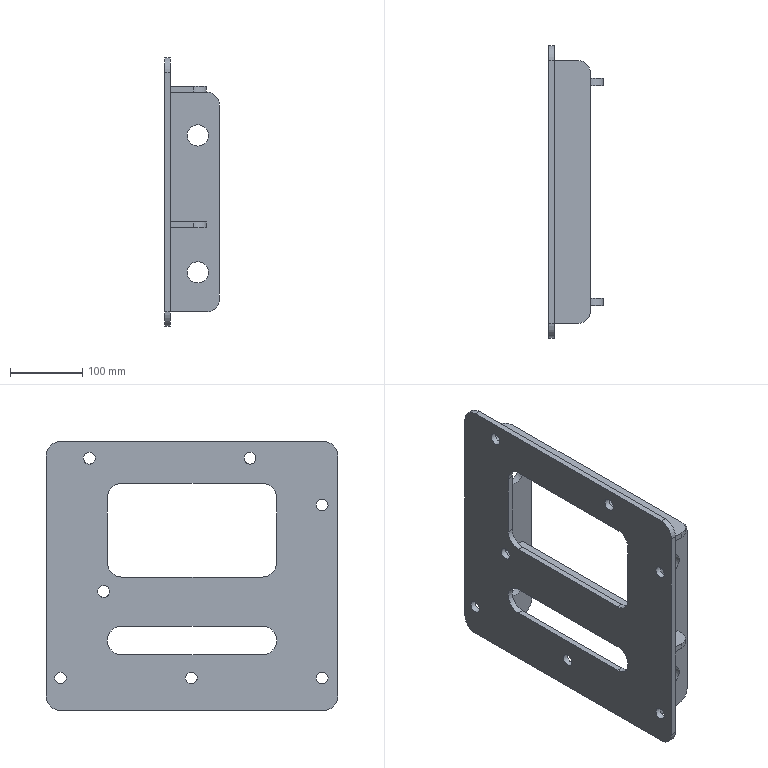Part | STEP file | HL4GZ-1.862.096 (cutter mechanism mounting seat weldment) | 7 solids | 77 faces | box 76 x 405 x 373 mm | volume 1546147 mm3 | plane 48 | cylinder 29 | commonest cylinder face diameters 40 x10 36 x8 16.5 x7 29.5 x4